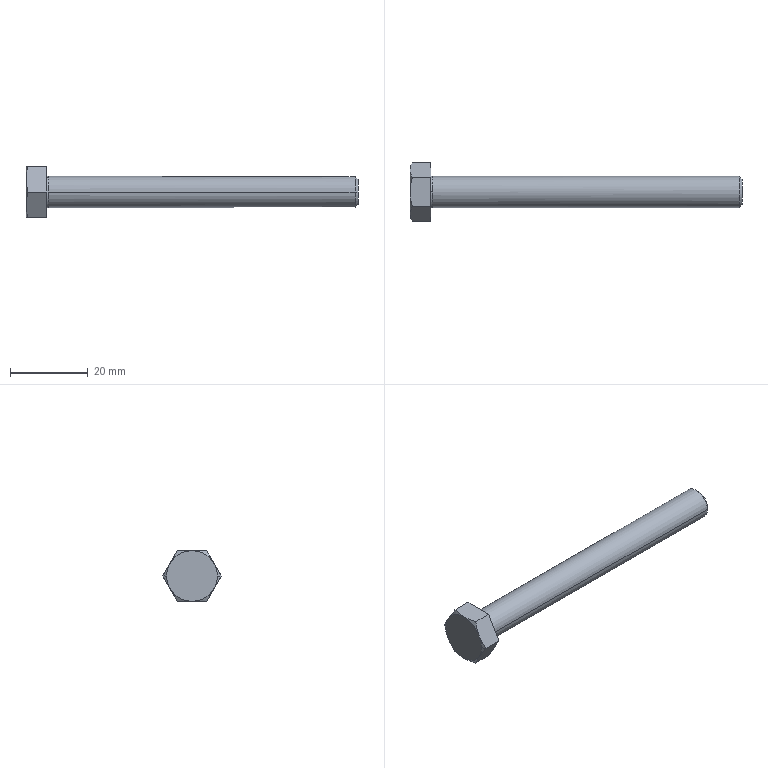Part | STEP file | KS B 1002 - C  M 8 x 80 | 1 solid | 23 faces | box 85.3 x 15.011 x 13 mm | volume 4789 mm3 | cone 10 | plane 9 | torus 2 | cylinder 2 | commonest cylinder face diameters 8 x2